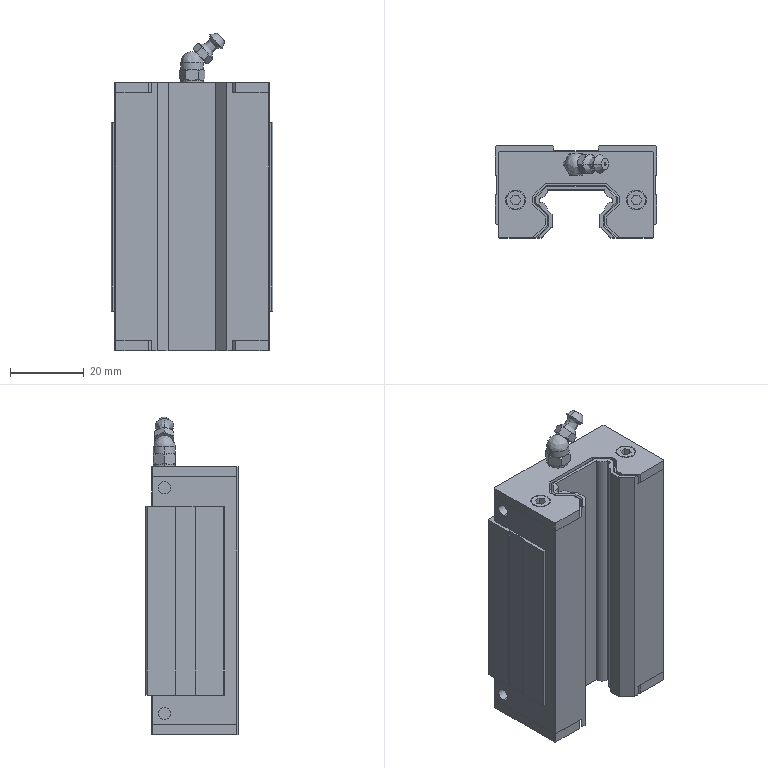Part | SolidWorks | features ICE 34, HoleWzd 8, Chamfer 4, BaseBody 1 | 1 solid | 299 faces | box 44 x 25 x 86.312 mm | volume 60891 mm3 | plane 213 | cylinder 44 | cone 39 | spline 3 | commonest cylinder face diameters 5 x16 3.3 x8 5.4 x8 4.455 x6 6 x4 0.8 x2